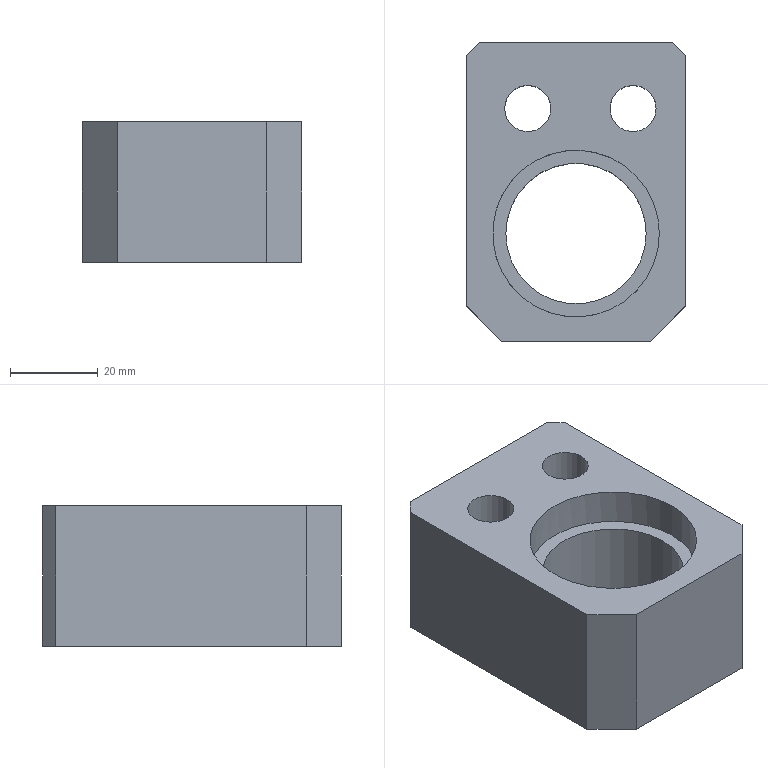Part | STEP file | lll_id3678_x_t | 1 solid | 19 faces | box 50 x 68 x 32 mm | volume 67708 mm3 | plane 13 | cylinder 6 | commonest cylinder face diameters 10.5 x2 17 x2 32 x1 38 x1
STEP:
#1=CARTESIAN_POINT('',(3219.117,232.788,77.5));
#2=VERTEX_POINT('',#1);
#3=CARTESIAN_POINT('',(3224.367,232.788,77.5));
#4=DIRECTION('',(0.,0.,1.));
#5=DIRECTION('',(-1.,0.,0.));
#6=AXIS2_PLACEMENT_3D('',#3,#4,#5);
#7=CIRCLE('',#6,5.25);
#8=EDGE_CURVE('',#2,#2,#7,.T.);
#9=ORIENTED_EDGE('',*,*,#8,.T.);
#10=EDGE_LOOP('',(#9));
#11=FACE_BOUND('',#10,.T.);
#12=CARTESIAN_POINT('',(3215.867,232.788,77.5));
#13=VERTEX_POINT('',#12);
#14=CARTESIAN_POINT('',(3224.367,232.788,77.5));
#15=DIRECTION('',(0.,0.,1.));
#16=DIRECTION('',(-1.,0.,0.));
#17=AXIS2_PLACEMENT_3D('',#14,#15,#16);
#18=CIRCLE('',#17,8.5);
#19=EDGE_CURVE('',#13,#13,#18,.T.);
#20=ORIENTED_EDGE('',*,*,#19,.F.);
#21=EDGE_LOOP('',(#20));
#22=FACE_BOUND('',#21,.T.);
#23=CARTESIAN_POINT('',(3224.367,232.788,77.5));
#24=DIRECTION('',(0.,0.,1.));
#25=DIRECTION('',(-1.,0.,0.));
#26=AXIS2_PLACEMENT_3D('',#23,#24,#25);
#27=PLANE('',#26);
#28=ADVANCED_FACE('',(#11,#22),#27,.F.);
#29=CARTESIAN_POINT('',(3216.367,204.288,84.3));
#30=VERTEX_POINT('',#29);
#31=CARTESIAN_POINT('',(3235.367,204.288,84.3));
#32=DIRECTION('',(0.,0.,1.));
#33=DIRECTION('',(-1.,0.,0.));
#34=AXIS2_PLACEMENT_3D('',#31,#32,#33);
#35=CIRCLE('',#34,19.);
#36=EDGE_CURVE('',#30,#30,#35,.T.);
#37=ORIENTED_EDGE('',*,*,#36,.T.);
#38=EDGE_LOOP('',(#37));
#39=FACE_BOUND('',#38,.T.);
#40=CARTESIAN_POINT('',(3219.367,204.288,84.3));
#41=VERTEX_POINT('',#40);
#42=CARTESIAN_POINT('',(3235.367,204.288,84.3));
#43=DIRECTION('',(0.,0.,1.));
#44=DIRECTION('',(-1.,0.,0.));
#45=AXIS2_PLACEMENT_3D('',#42,#43,#44);
#46=CIRCLE('',#45,16.);
#47=EDGE_CURVE('',#41,#41,#46,.T.);
#48=ORIENTED_EDGE('',*,*,#47,.F.);
#49=EDGE_LOOP('',(#48));
#50=FACE_BOUND('',#49,.T.);
#51=CARTESIAN_POINT('',(3235.367,213.038,84.3));
#52=DIRECTION('',(0.,0.,-1.));
#53=DIRECTION('',(0.,1.,0.));
#54=AXIS2_PLACEMENT_3D('',#51,#52,#53);
#55=PLANE('',#54);
#56=ADVANCED_FACE('',(#39,#50),#55,.F.);
#57=ORIENTED_EDGE('',*,*,#19,.T.);
#58=EDGE_LOOP('',(#57));
#59=FACE_BOUND('',#58,.T.);
#60=CARTESIAN_POINT('',(3215.867,232.788,60.5));
#61=VERTEX_POINT('',#60);
#62=CARTESIAN_POINT('',(3224.367,232.788,60.5));
#63=DIRECTION('',(0.,0.,-1.));
#64=DIRECTION('',(-1.,0.,0.));
#65=AXIS2_PLACEMENT_3D('',#62,#63,#64);
#66=CIRCLE('',#65,8.5);
#67=EDGE_CURVE('',#61,#61,#66,.T.);
#68=ORIENTED_EDGE('',*,*,#67,.T.);
#69=EDGE_LOOP('',(#68));
#70=FACE_BOUND('',#69,.T.);
#71=CARTESIAN_POINT('',(3224.367,232.788,60.5));
#72=DIRECTION('',(0.,0.,1.));
#73=DIRECTION('',(-1.,0.,0.));
#74=AXIS2_PLACEMENT_3D('',#71,#72,#73);
#75=CYLINDRICAL_SURFACE('',#74,8.5);
#76=ADVANCED_FACE('',(#59,#70),#75,.F.);
#77=CARTESIAN_POINT('',(3252.366,179.788,60.5));
#78=VERTEX_POINT('',#77);
#79=CARTESIAN_POINT('',(3218.367,179.788,60.5));
#80=VERTEX_POINT('',#79);
#81=CARTESIAN_POINT('',(3172.176,179.788,60.5));
#82=DIRECTION('',(-1.,0.,0.));
#83=VECTOR('',#82,1.);
#84=LINE('',#81,#83);
#85=EDGE_CURVE('',#78,#80,#84,.T.);
#86=ORIENTED_EDGE('',*,*,#85,.F.);
#87=CARTESIAN_POINT('',(3252.366,179.788,92.5));
#88=VERTEX_POINT('',#87);
#89=CARTESIAN_POINT('',(3252.366,179.788,-8.5));
#90=DIRECTION('',(0.,0.,1.));
#91=VECTOR('',#90,1.);
#92=LINE('',#89,#91);
#93=EDGE_CURVE('',#78,#88,#92,.T.);
#94=ORIENTED_EDGE('',*,*,#93,.T.);
#95=CARTESIAN_POINT('',(3218.367,179.788,92.5));
#96=VERTEX_POINT('',#95);
#97=CARTESIAN_POINT('',(3235.367,179.788,92.5));
#98=DIRECTION('',(1.,0.,0.));
#99=VECTOR('',#98,1.);
#100=LINE('',#97,#99);
#101=EDGE_CURVE('',#96,#88,#100,.T.);
#102=ORIENTED_EDGE('',*,*,#101,.F.);
#103=CARTESIAN_POINT('',(3218.367,179.788,-8.5));
#104=DIRECTION('',(0.,0.,-1.));
#105=VECTOR('',#104,1.);
#106=LINE('',#103,#105);
#107=EDGE_CURVE('',#96,#80,#106,.T.);
#108=ORIENTED_EDGE('',*,*,#107,.T.);
#109=EDGE_LOOP('',(#86,#94,#102,#108));
#110=FACE_OUTER_BOUND('',#109,.T.);
#111=CARTESIAN_POINT('',(3235.367,179.788,-8.5));
#112=DIRECTION('',(0.,-1.,0.));
#113=DIRECTION('',(0.,0.,-1.));
#114=AXIS2_PLACEMENT_3D('',#111,#112,#113);
#115=PLANE('',#114);
#116=ADVANCED_FACE('',(#110),#115,.T.);
#117=CARTESIAN_POINT('',(3210.367,244.788,92.5));
#118=VERTEX_POINT('',#117);
#119=CARTESIAN_POINT('',(3210.367,187.788,92.5));
#120=VERTEX_POINT('',#119);
#121=CARTESIAN_POINT('',(3210.367,235.513,92.5));
#122=DIRECTION('',(0.,-1.,0.));
#123=VECTOR('',#122,1.);
#124=LINE('',#121,#123);
#125=EDGE_CURVE('',#118,#120,#124,.T.);
#126=ORIENTED_EDGE('',*,*,#125,.F.);
#127=CARTESIAN_POINT('',(3210.367,244.788,60.5));
#128=VERTEX_POINT('',#127);
#129=CARTESIAN_POINT('',(3210.367,244.788,-8.5));
#130=DIRECTION('',(0.,0.,-1.));
#131=VECTOR('',#130,1.);
#132=LINE('',#129,#131);
#133=EDGE_CURVE('',#118,#128,#132,.T.);
#134=ORIENTED_EDGE('',*,*,#133,.T.);
#135=CARTESIAN_POINT('',(3210.367,187.788,60.5));
#136=VERTEX_POINT('',#135);
#137=CARTESIAN_POINT('',(3210.367,230.563,60.5));
#138=DIRECTION('',(0.,1.,0.));
#139=VECTOR('',#138,1.);
#140=LINE('',#137,#139);
#141=EDGE_CURVE('',#136,#128,#140,.T.);
#142=ORIENTED_EDGE('',*,*,#141,.F.);
#143=CARTESIAN_POINT('',(3210.367,187.788,-8.5));
#144=DIRECTION('',(0.,0.,1.));
#145=VECTOR('',#144,1.);
#146=LINE('',#143,#145);
#147=EDGE_CURVE('',#136,#120,#146,.T.);
#148=ORIENTED_EDGE('',*,*,#147,.T.);
#149=EDGE_LOOP('',(#126,#134,#142,#148));
#150=FACE_OUTER_BOUND('',#149,.T.);
#151=CARTESIAN_POINT('',(3210.367,204.288,-8.5));
#152=DIRECTION('',(-1.,0.,0.));
#153=DIRECTION('',(0.,0.,-1.));
#154=AXIS2_PLACEMENT_3D('',#151,#152,#153);
#155=PLANE('',#154);
#156=ADVANCED_FACE('',(#150),#155,.T.);
#157=CARTESIAN_POINT('',(3257.366,247.788,92.5));
#158=VERTEX_POINT('',#157);
#159=CARTESIAN_POINT('',(3213.367,247.788,92.5));
#160=VERTEX_POINT('',#159);
#161=CARTESIAN_POINT('',(3235.367,247.788,92.5));
#162=DIRECTION('',(-1.,0.,0.));
#163=VECTOR('',#162,1.);
#164=LINE('',#161,#163);
#165=EDGE_CURVE('',#158,#160,#164,.T.);
#166=ORIENTED_EDGE('',*,*,#165,.F.);
#167=CARTESIAN_POINT('',(3257.366,247.788,60.5));
#168=VERTEX_POINT('',#167);
#169=CARTESIAN_POINT('',(3257.366,247.788,-8.5));
#170=DIRECTION('',(0.,0.,-1.));
#171=VECTOR('',#170,1.);
#172=LINE('',#169,#171);
#173=EDGE_CURVE('',#158,#168,#172,.T.);
#174=ORIENTED_EDGE('',*,*,#173,.T.);
#175=CARTESIAN_POINT('',(3213.367,247.788,60.5));
#176=VERTEX_POINT('',#175);
#177=CARTESIAN_POINT('',(3172.176,247.788,60.5));
#178=DIRECTION('',(1.,0.,0.));
#179=VECTOR('',#178,1.);
#180=LINE('',#177,#179);
#181=EDGE_CURVE('',#176,#168,#180,.T.);
#182=ORIENTED_EDGE('',*,*,#181,.F.);
#183=CARTESIAN_POINT('',(3213.367,247.788,-8.5));
#184=DIRECTION('',(0.,0.,1.));
#185=VECTOR('',#184,1.);
#186=LINE('',#183,#185);
#187=EDGE_CURVE('',#176,#160,#186,.T.);
#188=ORIENTED_EDGE('',*,*,#187,.T.);
#189=EDGE_LOOP('',(#166,#174,#182,#188));
#190=FACE_OUTER_BOUND('',#189,.T.);
#191=CARTESIAN_POINT('',(3235.367,247.788,-8.5));
#192=DIRECTION('',(0.,1.,0.));
#193=DIRECTION('',(0.,0.,1.));
#194=AXIS2_PLACEMENT_3D('',#191,#192,#193);
#195=PLANE('',#194);
#196=ADVANCED_FACE('',(#190),#195,.T.);
#197=CARTESIAN_POINT('',(3260.366,244.788,60.5));
#198=VERTEX_POINT('',#197);
#199=CARTESIAN_POINT('',(3260.366,187.788,60.5));
#200=VERTEX_POINT('',#199);
#201=CARTESIAN_POINT('',(3260.366,230.563,60.5));
#202=DIRECTION('',(0.,-1.,0.));
#203=VECTOR('',#202,1.);
#204=LINE('',#201,#203);
#205=EDGE_CURVE('',#198,#200,#204,.T.);
#206=ORIENTED_EDGE('',*,*,#205,.F.);
#207=CARTESIAN_POINT('',(3260.366,244.788,92.5));
#208=VERTEX_POINT('',#207);
#209=CARTESIAN_POINT('',(3260.366,244.788,-8.5));
#210=DIRECTION('',(0.,0.,1.));
#211=VECTOR('',#210,1.);
#212=LINE('',#209,#211);
#213=EDGE_CURVE('',#198,#208,#212,.T.);
#214=ORIENTED_EDGE('',*,*,#213,.T.);
#215=CARTESIAN_POINT('',(3260.366,187.788,92.5));
#216=VERTEX_POINT('',#215);
#217=CARTESIAN_POINT('',(3260.366,230.563,92.5));
#218=DIRECTION('',(0.,1.,0.));
#219=VECTOR('',#218,1.);
#220=LINE('',#217,#219);
#221=EDGE_CURVE('',#216,#208,#220,.T.);
#222=ORIENTED_EDGE('',*,*,#221,.F.);
#223=CARTESIAN_POINT('',(3260.366,187.788,-8.5));
#224=DIRECTION('',(0.,0.,-1.));
#225=VECTOR('',#224,1.);
#226=LINE('',#223,#225);
#227=EDGE_CURVE('',#216,#200,#226,.T.);
#228=ORIENTED_EDGE('',*,*,#227,.T.);
#229=EDGE_LOOP('',(#206,#214,#222,#228));
#230=FACE_OUTER_BOUND('',#229,.T.);
#231=CARTESIAN_POINT('',(3260.366,199.338,-8.5));
#232=DIRECTION('',(1.,0.,0.));
#233=DIRECTION('',(0.,0.,1.));
#234=AXIS2_PLACEMENT_3D('',#231,#232,#233);
#235=PLANE('',#234);
#236=ADVANCED_FACE('',(#230),#235,.T.);
#237=CARTESIAN_POINT('',(3219.117,232.788,92.5));
#238=VERTEX_POINT('',#237);
#239=CARTESIAN_POINT('',(3224.367,232.788,92.5));
#240=DIRECTION('',(0.,0.,-1.));
#241=DIRECTION('',(-1.,0.,0.));
#242=AXIS2_PLACEMENT_3D('',#239,#240,#241);
#243=CIRCLE('',#242,5.25);
#244=EDGE_CURVE('',#238,#238,#243,.T.);
#245=ORIENTED_EDGE('',*,*,#244,.F.);
#246=EDGE_LOOP('',(#245));
#247=FACE_BOUND('',#246,.T.);
#248=ORIENTED_EDGE('',*,*,#8,.F.);
#249=EDGE_LOOP('',(#248));
#250=FACE_BOUND('',#249,.T.);
#251=CARTESIAN_POINT('',(3224.367,232.788,160.5));
#252=DIRECTION('',(0.,0.,1.));
#253=DIRECTION('',(-1.,0.,0.));
#254=AXIS2_PLACEMENT_3D('',#251,#252,#253);
#255=CYLINDRICAL_SURFACE('',#254,5.25);
#256=ADVANCED_FACE('',(#247,#250),#255,.F.);
#257=CARTESIAN_POINT('',(3254.367,204.288,92.5));
#258=VERTEX_POINT('',#257);
#259=CARTESIAN_POINT('',(3235.367,204.288,92.5));
#260=DIRECTION('',(0.,0.,-1.));
#261=DIRECTION('',(1.,0.,0.));
#262=AXIS2_PLACEMENT_3D('',#259,#260,#261);
#263=CIRCLE('',#262,19.);
#264=EDGE_CURVE('',#258,#258,#263,.T.);
#265=ORIENTED_EDGE('',*,*,#264,.F.);
#266=EDGE_LOOP('',(#265));
#267=FACE_BOUND('',#266,.T.);
#268=ORIENTED_EDGE('',*,*,#36,.F.);
#269=EDGE_LOOP('',(#268));
#270=FACE_BOUND('',#269,.T.);
#271=CARTESIAN_POINT('',(3235.367,204.288,90.));
#272=DIRECTION('',(0.,0.,-1.));
#273=DIRECTION('',(0.,-1.,0.));
#274=AXIS2_PLACEMENT_3D('',#271,#272,#273);
#275=CYLINDRICAL_SURFACE('',#274,19.);
#276=ADVANCED_FACE('',(#267,#270),#275,.F.);
#277=CARTESIAN_POINT('',(3253.617,232.788,92.5));
#278=VERTEX_POINT('',#277);
#279=CARTESIAN_POINT('',(3248.367,232.788,92.5));
#280=DIRECTION('',(0.,0.,1.));
#281=DIRECTION('',(1.,0.,0.));
#282=AXIS2_PLACEMENT_3D('',#279,#280,#281);
#283=CIRCLE('',#282,5.25);
#284=EDGE_CURVE('',#278,#278,#283,.T.);
#285=ORIENTED_EDGE('',*,*,#284,.F.);
#286=EDGE_LOOP('',(#285));
#287=FACE_BOUND('',#286,.T.);
#288=ORIENTED_EDGE('',*,*,#264,.T.);
#289=EDGE_LOOP('',(#288));
#290=FACE_BOUND('',#289,.T.);
#291=ORIENTED_EDGE('',*,*,#244,.T.);
#292=EDGE_LOOP('',(#291));
#293=FACE_BOUND('',#292,.T.);
#294=ORIENTED_EDGE('',*,*,#221,.T.);
#295=CARTESIAN_POINT('',(3218.434,286.72,92.5));
#296=DIRECTION('',(-0.7071,0.7071,0.));
#297=VECTOR('',#296,1.);
#298=LINE('',#295,#297);
#299=EDGE_CURVE('',#208,#158,#298,.T.);
#300=ORIENTED_EDGE('',*,*,#299,.T.);
#301=ORIENTED_EDGE('',*,*,#165,.T.);
#302=CARTESIAN_POINT('',(3184.159,218.58,92.5));
#303=DIRECTION('',(-0.7071,-0.7071,0.));
#304=VECTOR('',#303,1.);
#305=LINE('',#302,#304);
#306=EDGE_CURVE('',#160,#118,#305,.T.);
#307=ORIENTED_EDGE('',*,*,#306,.T.);
#308=ORIENTED_EDGE('',*,*,#125,.T.);
#309=CARTESIAN_POINT('',(3164.934,233.22,92.5));
#310=DIRECTION('',(0.7071,-0.7071,0.));
#311=VECTOR('',#310,1.);
#312=LINE('',#309,#311);
#313=EDGE_CURVE('',#120,#96,#312,.T.);
#314=ORIENTED_EDGE('',*,*,#313,.T.);
#315=ORIENTED_EDGE('',*,*,#101,.T.);
#316=CARTESIAN_POINT('',(3237.659,165.08,92.5));
#317=DIRECTION('',(0.7071,0.7071,0.));
#318=VECTOR('',#317,1.);
#319=LINE('',#316,#318);
#320=EDGE_CURVE('',#88,#216,#319,.T.);
#321=ORIENTED_EDGE('',*,*,#320,.T.);
#322=EDGE_LOOP('',(#294,#300,#301,#307,#308,#314,#315,#321));
#323=FACE_BOUND('',#322,.T.);
#324=CARTESIAN_POINT('',(3167.227,235.513,92.5));
#325=DIRECTION('',(0.,0.,1.));
#326=DIRECTION('',(-1.,0.,0.));
#327=AXIS2_PLACEMENT_3D('',#324,#325,#326);
#328=PLANE('',#327);
#329=ADVANCED_FACE('',(#287,#290,#293,#323),#328,.T.);
#330=CARTESIAN_POINT('',(3251.367,204.288,60.5));
#331=VERTEX_POINT('',#330);
#332=CARTESIAN_POINT('',(3235.367,204.288,60.5));
#333=DIRECTION('',(0.,0.,1.));
#334=DIRECTION('',(1.,0.,0.));
#335=AXIS2_PLACEMENT_3D('',#332,#333,#334);
#336=CIRCLE('',#335,16.);
#337=EDGE_CURVE('',#331,#331,#336,.T.);
#338=ORIENTED_EDGE('',*,*,#337,.F.);
#339=EDGE_LOOP('',(#338));
#340=FACE_BOUND('',#339,.T.);
#341=ORIENTED_EDGE('',*,*,#47,.T.);
#342=EDGE_LOOP('',(#341));
#343=FACE_BOUND('',#342,.T.);
#344=CARTESIAN_POINT('',(3235.367,204.288,44.8));
#345=DIRECTION('',(0.,0.,-1.));
#346=DIRECTION('',(0.,-1.,0.));
#347=AXIS2_PLACEMENT_3D('',#344,#345,#346);
#348=CYLINDRICAL_SURFACE('',#347,16.);
#349=ADVANCED_FACE('',(#340,#343),#348,.F.);
#350=CARTESIAN_POINT('',(3256.867,232.788,60.5));
#351=VERTEX_POINT('',#350);
#352=CARTESIAN_POINT('',(3248.367,232.788,60.5));
#353=DIRECTION('',(0.,0.,-1.));
#354=DIRECTION('',(1.,0.,0.));
#355=AXIS2_PLACEMENT_3D('',#352,#353,#354);
#356=CIRCLE('',#355,8.5);
#357=EDGE_CURVE('',#351,#351,#356,.T.);
#358=ORIENTED_EDGE('',*,*,#357,.F.);
#359=EDGE_LOOP('',(#358));
#360=FACE_BOUND('',#359,.T.);
#361=ORIENTED_EDGE('',*,*,#337,.T.);
#362=EDGE_LOOP('',(#361));
#363=FACE_BOUND('',#362,.T.);
#364=ORIENTED_EDGE('',*,*,#181,.T.);
#365=CARTESIAN_POINT('',(3223.383,281.771,60.5));
#366=DIRECTION('',(0.7071,-0.7071,0.));
#367=VECTOR('',#366,1.);
#368=LINE('',#365,#367);
#369=EDGE_CURVE('',#168,#198,#368,.T.);
#370=ORIENTED_EDGE('',*,*,#369,.T.);
#371=ORIENTED_EDGE('',*,*,#205,.T.);
#372=CARTESIAN_POINT('',(3237.659,165.08,60.5));
#373=DIRECTION('',(-0.7071,-0.7071,0.));
#374=VECTOR('',#373,1.);
#375=LINE('',#372,#374);
#376=EDGE_CURVE('',#200,#78,#375,.T.);
#377=ORIENTED_EDGE('',*,*,#376,.T.);
#378=ORIENTED_EDGE('',*,*,#85,.T.);
#379=CARTESIAN_POINT('',(3169.884,228.271,60.5));
#380=DIRECTION('',(-0.7071,0.7071,0.));
#381=VECTOR('',#380,1.);
#382=LINE('',#379,#381);
#383=EDGE_CURVE('',#80,#136,#382,.T.);
#384=ORIENTED_EDGE('',*,*,#383,.T.);
#385=ORIENTED_EDGE('',*,*,#141,.T.);
#386=CARTESIAN_POINT('',(3184.159,218.58,60.5));
#387=DIRECTION('',(0.7071,0.7071,0.));
#388=VECTOR('',#387,1.);
#389=LINE('',#386,#388);
#390=EDGE_CURVE('',#128,#176,#389,.T.);
#391=ORIENTED_EDGE('',*,*,#390,.T.);
#392=EDGE_LOOP('',(#364,#370,#371,#377,#378,#384,#385,#391));
#393=FACE_BOUND('',#392,.T.);
#394=ORIENTED_EDGE('',*,*,#67,.F.);
#395=EDGE_LOOP('',(#394));
#396=FACE_BOUND('',#395,.T.);
#397=CARTESIAN_POINT('',(3172.176,230.563,60.5));
#398=DIRECTION('',(0.,0.,1.));
#399=DIRECTION('',(-1.,0.,0.));
#400=AXIS2_PLACEMENT_3D('',#397,#398,#399);
#401=PLANE('',#400);
#402=ADVANCED_FACE('',(#360,#363,#393,#396),#401,.F.);
#403=CARTESIAN_POINT('',(3243.117,232.788,77.5));
#404=VERTEX_POINT('',#403);
#405=CARTESIAN_POINT('',(3248.367,232.788,77.5));
#406=DIRECTION('',(0.,0.,1.));
#407=DIRECTION('',(-1.,0.,0.));
#408=AXIS2_PLACEMENT_3D('',#405,#406,#407);
#409=CIRCLE('',#408,5.25);
#410=EDGE_CURVE('',#404,#404,#409,.T.);
#411=ORIENTED_EDGE('',*,*,#410,.T.);
#412=EDGE_LOOP('',(#411));
#413=FACE_BOUND('',#412,.T.);
#414=CARTESIAN_POINT('',(3239.867,232.788,77.5));
#415=VERTEX_POINT('',#414);
#416=CARTESIAN_POINT('',(3248.367,232.788,77.5));
#417=DIRECTION('',(0.,0.,1.));
#418=DIRECTION('',(-1.,0.,0.));
#419=AXIS2_PLACEMENT_3D('',#416,#417,#418);
#420=CIRCLE('',#419,8.5);
#421=EDGE_CURVE('',#415,#415,#420,.T.);
#422=ORIENTED_EDGE('',*,*,#421,.F.);
#423=EDGE_LOOP('',(#422));
#424=FACE_BOUND('',#423,.T.);
#425=CARTESIAN_POINT('',(3248.367,232.788,77.5));
#426=DIRECTION('',(0.,0.,1.));
#427=DIRECTION('',(-1.,0.,0.));
#428=AXIS2_PLACEMENT_3D('',#425,#426,#427);
#429=PLANE('',#428);
#430=ADVANCED_FACE('',(#413,#424),#429,.F.);
#431=ORIENTED_EDGE('',*,*,#284,.T.);
#432=EDGE_LOOP('',(#431));
#433=FACE_BOUND('',#432,.T.);
#434=ORIENTED_EDGE('',*,*,#410,.F.);
#435=EDGE_LOOP('',(#434));
#436=FACE_BOUND('',#435,.T.);
#437=CARTESIAN_POINT('',(3248.367,232.788,160.5));
#438=DIRECTION('',(0.,0.,1.));
#439=DIRECTION('',(-1.,0.,0.));
#440=AXIS2_PLACEMENT_3D('',#437,#438,#439);
#441=CYLINDRICAL_SURFACE('',#440,5.25);
#442=ADVANCED_FACE('',(#433,#436),#441,.F.);
#443=ORIENTED_EDGE('',*,*,#421,.T.);
#444=EDGE_LOOP('',(#443));
#445=FACE_BOUND('',#444,.T.);
#446=ORIENTED_EDGE('',*,*,#357,.T.);
#447=EDGE_LOOP('',(#446));
#448=FACE_BOUND('',#447,.T.);
#449=CARTESIAN_POINT('',(3248.367,232.788,60.5));
#450=DIRECTION('',(0.,0.,1.));
#451=DIRECTION('',(-1.,0.,0.));
#452=AXIS2_PLACEMENT_3D('',#449,#450,#451);
#453=CYLINDRICAL_SURFACE('',#452,8.5);
#454=ADVANCED_FACE('',(#445,#448),#453,.F.);
#455=ORIENTED_EDGE('',*,*,#320,.F.);
#456=ORIENTED_EDGE('',*,*,#93,.F.);
#457=ORIENTED_EDGE('',*,*,#376,.F.);
#458=ORIENTED_EDGE('',*,*,#227,.F.);
#459=EDGE_LOOP('',(#455,#456,#457,#458));
#460=FACE_OUTER_BOUND('',#459,.T.);
#461=CARTESIAN_POINT('',(3260.366,187.788,-8.5));
#462=DIRECTION('',(-0.7071,0.7071,0.));
#463=DIRECTION('',(0.,0.,-1.));
#464=AXIS2_PLACEMENT_3D('',#461,#462,#463);
#465=PLANE('',#464);
#466=ADVANCED_FACE('',(#460),#465,.F.);
#467=ORIENTED_EDGE('',*,*,#383,.F.);
#468=ORIENTED_EDGE('',*,*,#107,.F.);
#469=ORIENTED_EDGE('',*,*,#313,.F.);
#470=ORIENTED_EDGE('',*,*,#147,.F.);
#471=EDGE_LOOP('',(#467,#468,#469,#470));
#472=FACE_OUTER_BOUND('',#471,.T.);
#473=CARTESIAN_POINT('',(3210.367,187.788,-8.5));
#474=DIRECTION('',(0.7071,0.7071,0.));
#475=DIRECTION('',(0.,0.,1.));
#476=AXIS2_PLACEMENT_3D('',#473,#474,#475);
#477=PLANE('',#476);
#478=ADVANCED_FACE('',(#472),#477,.F.);
#479=ORIENTED_EDGE('',*,*,#369,.F.);
#480=ORIENTED_EDGE('',*,*,#173,.F.);
#481=ORIENTED_EDGE('',*,*,#299,.F.);
#482=ORIENTED_EDGE('',*,*,#213,.F.);
#483=EDGE_LOOP('',(#479,#480,#481,#482));
#484=FACE_OUTER_BOUND('',#483,.T.);
#485=CARTESIAN_POINT('',(3260.366,244.788,-8.5));
#486=DIRECTION('',(-0.7071,-0.7071,0.));
#487=DIRECTION('',(0.,0.,1.));
#488=AXIS2_PLACEMENT_3D('',#485,#486,#487);
#489=PLANE('',#488);
#490=ADVANCED_FACE('',(#484),#489,.F.);
#491=ORIENTED_EDGE('',*,*,#390,.F.);
#492=ORIENTED_EDGE('',*,*,#133,.F.);
#493=ORIENTED_EDGE('',*,*,#306,.F.);
#494=ORIENTED_EDGE('',*,*,#187,.F.);
#495=EDGE_LOOP('',(#491,#492,#493,#494));
#496=FACE_OUTER_BOUND('',#495,.T.);
#497=CARTESIAN_POINT('',(3213.367,247.788,-8.5));
#498=DIRECTION('',(0.7071,-0.7071,0.));
#499=DIRECTION('',(0.,0.,1.));
#500=AXIS2_PLACEMENT_3D('',#497,#498,#499);
#501=PLANE('',#500);
#502=ADVANCED_FACE('',(#496),#501,.F.);
#503=CLOSED_SHELL('',(#28,#56,#76,#116,#156,#196,#236,#256,#276,#329,#349,#402,#430,#442,#454,#466,#478,#490,#502));
#504=MANIFOLD_SOLID_BREP('',#503);
#505=(LENGTH_UNIT()NAMED_UNIT(*)SI_UNIT(.MILLI.,.METRE.));
#506=UNCERTAINTY_MEASURE_WITH_UNIT(LENGTH_MEASURE(0.00002),#505,'','');
#507=(NAMED_UNIT(*)PLANE_ANGLE_UNIT()SI_UNIT($,.RADIAN.));
#508=PLANE_ANGLE_MEASURE_WITH_UNIT(PLANE_ANGLE_MEASURE(0.01745),#507);
#509=DIMENSIONAL_EXPONENTS(0.,0.,0.,0.,0.,0.,0.);
#510=(CONVERSION_BASED_UNIT('DEGREE',#508)NAMED_UNIT(#509)PLANE_ANGLE_UNIT());
#511=(NAMED_UNIT(*)SI_UNIT($,.STERADIAN.)SOLID_ANGLE_UNIT());
#512=(GEOMETRIC_REPRESENTATION_CONTEXT(3)GLOBAL_UNCERTAINTY_ASSIGNED_CONTEXT((#506))GLOBAL_UNIT_ASSIGNED_CONTEXT((#505,#510,#511))REPRESENTATION_CONTEXT('',''));
#513=ADVANCED_BREP_SHAPE_REPRESENTATION('',(#504),#512);